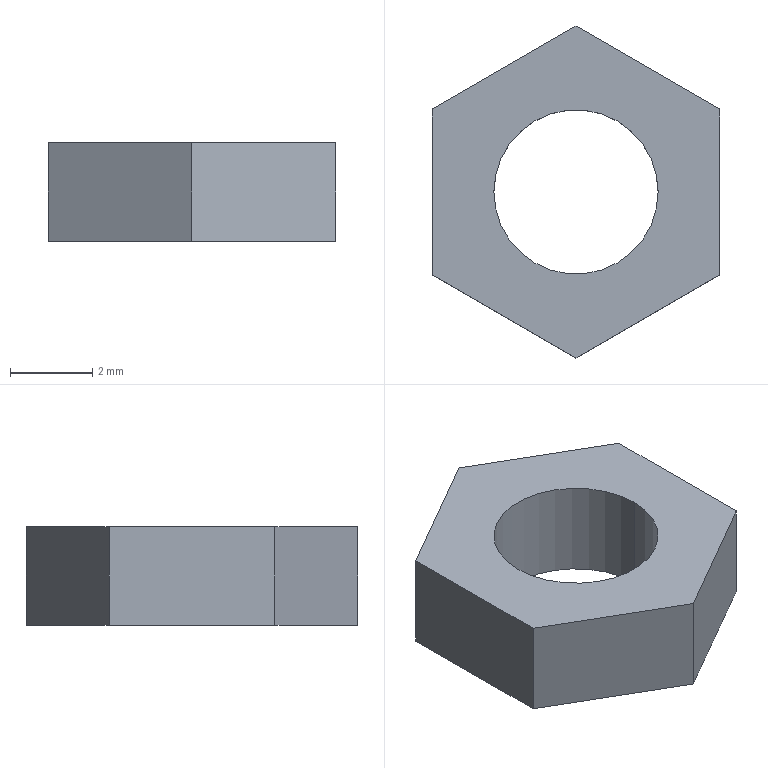Part | STEP file | M4 nut | 1 solid | 10 faces | box 7 x 8.083 x 2.4 mm | volume 71.685 mm3 | plane 8 | cylinder 2 | commonest cylinder face diameters 4 x2
STEP:
#1=CARTESIAN_POINT('',(0.,0.,0.));
#2=DIRECTION('',(0.,0.,1.));
#3=DIRECTION('',(1.,0.,0.));
#4=AXIS2_PLACEMENT_3D('',#1,#2,#3);
#5=CARTESIAN_POINT('',(2.,0.,0.));
#6=VERTEX_POINT('',#5);
#7=CARTESIAN_POINT('',(2.,0.,2.4));
#8=VERTEX_POINT('',#7);
#9=CARTESIAN_POINT('',(2.,0.,0.));
#10=DIRECTION('',(0.,0.,1.));
#11=VECTOR('',#10,1.);
#12=LINE('',#9,#11);
#13=CARTESIAN_POINT('',(0.,0.,0.));
#14=DIRECTION('',(0.,0.,1.));
#15=DIRECTION('',(1.,0.,0.));
#16=AXIS2_PLACEMENT_3D('',#13,#14,#15);
#17=CYLINDRICAL_SURFACE('',#16,2.);
#18=CARTESIAN_POINT('',(6.283,0.));
#19=DIRECTION('',(0.,1.));
#20=VECTOR('',#19,1.);
#21=LINE('',#18,#20);
#22=(GEOMETRIC_REPRESENTATION_CONTEXT(2)PARAMETRIC_REPRESENTATION_CONTEXT()REPRESENTATION_CONTEXT('',''));
#23=DEFINITIONAL_REPRESENTATION('',(#21),#22);
#24=PCURVE('',#17,#23);
#25=CARTESIAN_POINT('',(0.,0.,0.));
#26=DIRECTION('',(0.,0.,1.));
#27=DIRECTION('',(1.,0.,0.));
#28=AXIS2_PLACEMENT_3D('',#25,#26,#27);
#29=CYLINDRICAL_SURFACE('',#28,2.);
#30=CARTESIAN_POINT('',(0.,0.));
#31=DIRECTION('',(0.,1.));
#32=VECTOR('',#31,1.);
#33=LINE('',#30,#32);
#34=(GEOMETRIC_REPRESENTATION_CONTEXT(2)PARAMETRIC_REPRESENTATION_CONTEXT()REPRESENTATION_CONTEXT('',''));
#35=DEFINITIONAL_REPRESENTATION('',(#33),#34);
#36=PCURVE('',#29,#35);
#37=SURFACE_CURVE('',#12,(#24,#36),.PCURVE_S1.);
#38=EDGE_CURVE('',#6,#8,#37,.T.);
#39=ORIENTED_EDGE('',*,*,#38,.T.);
#40=CARTESIAN_POINT('',(-2.,0.,2.4));
#41=VERTEX_POINT('',#40);
#42=CARTESIAN_POINT('',(0.,0.,2.4));
#43=DIRECTION('',(0.,0.,1.));
#44=DIRECTION('',(1.,0.,0.));
#45=AXIS2_PLACEMENT_3D('',#42,#43,#44);
#46=CIRCLE('',#45,2.);
#47=CARTESIAN_POINT('',(0.,2.4));
#48=DIRECTION('',(1.,0.));
#49=VECTOR('',#48,1.);
#50=LINE('',#47,#49);
#51=(GEOMETRIC_REPRESENTATION_CONTEXT(2)PARAMETRIC_REPRESENTATION_CONTEXT()REPRESENTATION_CONTEXT('',''));
#52=DEFINITIONAL_REPRESENTATION('',(#50),#51);
#53=PCURVE('',#17,#52);
#54=CARTESIAN_POINT('',(0.,0.,2.4));
#55=DIRECTION('',(0.,0.,1.));
#56=DIRECTION('',(1.,0.,0.));
#57=AXIS2_PLACEMENT_3D('',#54,#55,#56);
#58=PLANE('',#57);
#59=CARTESIAN_POINT('',(0.,0.));
#60=DIRECTION('',(1.,0.));
#61=AXIS2_PLACEMENT_2D('',#59,#60);
#62=CIRCLE('',#61,2.);
#63=(GEOMETRIC_REPRESENTATION_CONTEXT(2)PARAMETRIC_REPRESENTATION_CONTEXT()REPRESENTATION_CONTEXT('',''));
#64=DEFINITIONAL_REPRESENTATION('',(#62),#63);
#65=PCURVE('',#58,#64);
#66=SURFACE_CURVE('',#46,(#53,#65),.PCURVE_S1.);
#67=EDGE_CURVE('',#41,#8,#66,.T.);
#68=ORIENTED_EDGE('',*,*,#67,.F.);
#69=CARTESIAN_POINT('',(-2.,0.,0.));
#70=VERTEX_POINT('',#69);
#71=CARTESIAN_POINT('',(-2.,0.,0.));
#72=DIRECTION('',(0.,0.,1.));
#73=VECTOR('',#72,1.);
#74=LINE('',#71,#73);
#75=CARTESIAN_POINT('',(3.142,0.));
#76=DIRECTION('',(0.,1.));
#77=VECTOR('',#76,1.);
#78=LINE('',#75,#77);
#79=(GEOMETRIC_REPRESENTATION_CONTEXT(2)PARAMETRIC_REPRESENTATION_CONTEXT()REPRESENTATION_CONTEXT('',''));
#80=DEFINITIONAL_REPRESENTATION('',(#78),#79);
#81=PCURVE('',#17,#80);
#82=CARTESIAN_POINT('',(3.142,0.));
#83=DIRECTION('',(0.,1.));
#84=VECTOR('',#83,1.);
#85=LINE('',#82,#84);
#86=(GEOMETRIC_REPRESENTATION_CONTEXT(2)PARAMETRIC_REPRESENTATION_CONTEXT()REPRESENTATION_CONTEXT('',''));
#87=DEFINITIONAL_REPRESENTATION('',(#85),#86);
#88=PCURVE('',#29,#87);
#89=SURFACE_CURVE('',#74,(#81,#88),.PCURVE_S1.);
#90=EDGE_CURVE('',#70,#41,#89,.T.);
#91=ORIENTED_EDGE('',*,*,#90,.F.);
#92=CARTESIAN_POINT('',(0.,0.,0.));
#93=DIRECTION('',(0.,0.,1.));
#94=DIRECTION('',(1.,0.,0.));
#95=AXIS2_PLACEMENT_3D('',#92,#93,#94);
#96=CIRCLE('',#95,2.);
#97=CARTESIAN_POINT('',(0.,0.));
#98=DIRECTION('',(1.,0.));
#99=VECTOR('',#98,1.);
#100=LINE('',#97,#99);
#101=(GEOMETRIC_REPRESENTATION_CONTEXT(2)PARAMETRIC_REPRESENTATION_CONTEXT()REPRESENTATION_CONTEXT('',''));
#102=DEFINITIONAL_REPRESENTATION('',(#100),#101);
#103=PCURVE('',#17,#102);
#104=CARTESIAN_POINT('',(0.,0.,0.));
#105=DIRECTION('',(0.,0.,1.));
#106=DIRECTION('',(1.,0.,0.));
#107=AXIS2_PLACEMENT_3D('',#104,#105,#106);
#108=PLANE('',#107);
#109=CARTESIAN_POINT('',(0.,0.));
#110=DIRECTION('',(1.,0.));
#111=AXIS2_PLACEMENT_2D('',#109,#110);
#112=CIRCLE('',#111,2.);
#113=(GEOMETRIC_REPRESENTATION_CONTEXT(2)PARAMETRIC_REPRESENTATION_CONTEXT()REPRESENTATION_CONTEXT('',''));
#114=DEFINITIONAL_REPRESENTATION('',(#112),#113);
#115=PCURVE('',#108,#114);
#116=SURFACE_CURVE('',#96,(#103,#115),.PCURVE_S1.);
#117=EDGE_CURVE('',#70,#6,#116,.T.);
#118=ORIENTED_EDGE('',*,*,#117,.T.);
#119=EDGE_LOOP('',(#39,#68,#91,#118));
#120=FACE_BOUND('',#119,.F.);
#121=ADVANCED_FACE('',(#120),#17,.F.);
#122=CARTESIAN_POINT('',(-3.5,2.021,0.));
#123=VERTEX_POINT('',#122);
#124=CARTESIAN_POINT('',(-3.5,-2.021,0.));
#125=VERTEX_POINT('',#124);
#126=CARTESIAN_POINT('',(-3.5,2.021,0.));
#127=DIRECTION('',(0.,-1.,0.));
#128=VECTOR('',#127,1.);
#129=LINE('',#126,#128);
#130=CARTESIAN_POINT('',(-3.5,2.021,2.4));
#131=DIRECTION('',(1.,0.,0.));
#132=DIRECTION('',(0.,1.,0.));
#133=AXIS2_PLACEMENT_3D('',#130,#131,#132);
#134=PLANE('',#133);
#135=CARTESIAN_POINT('',(0.,-2.4));
#136=DIRECTION('',(-1.,0.));
#137=VECTOR('',#136,1.);
#138=LINE('',#135,#137);
#139=(GEOMETRIC_REPRESENTATION_CONTEXT(2)PARAMETRIC_REPRESENTATION_CONTEXT()REPRESENTATION_CONTEXT('',''));
#140=DEFINITIONAL_REPRESENTATION('',(#138),#139);
#141=PCURVE('',#134,#140);
#142=CARTESIAN_POINT('',(-3.5,2.021));
#143=DIRECTION('',(0.,-1.));
#144=VECTOR('',#143,1.);
#145=LINE('',#142,#144);
#146=(GEOMETRIC_REPRESENTATION_CONTEXT(2)PARAMETRIC_REPRESENTATION_CONTEXT()REPRESENTATION_CONTEXT('',''));
#147=DEFINITIONAL_REPRESENTATION('',(#145),#146);
#148=PCURVE('',#108,#147);
#149=SURFACE_CURVE('',#129,(#141,#148),.PCURVE_S1.);
#150=EDGE_CURVE('',#123,#125,#149,.T.);
#151=ORIENTED_EDGE('',*,*,#150,.T.);
#152=CARTESIAN_POINT('',(-3.5,-2.021,2.4));
#153=VERTEX_POINT('',#152);
#154=CARTESIAN_POINT('',(-3.5,-2.021,2.4));
#155=DIRECTION('',(0.,0.,-1.));
#156=VECTOR('',#155,1.);
#157=LINE('',#154,#156);
#158=CARTESIAN_POINT('',(-4.041,0.));
#159=DIRECTION('',(0.,-1.));
#160=VECTOR('',#159,1.);
#161=LINE('',#158,#160);
#162=(GEOMETRIC_REPRESENTATION_CONTEXT(2)PARAMETRIC_REPRESENTATION_CONTEXT()REPRESENTATION_CONTEXT('',''));
#163=DEFINITIONAL_REPRESENTATION('',(#161),#162);
#164=PCURVE('',#134,#163);
#165=CARTESIAN_POINT('',(-3.5,-2.021,2.4));
#166=DIRECTION('',(0.5,0.866,0.));
#167=DIRECTION('',(-0.866,0.5,0.));
#168=AXIS2_PLACEMENT_3D('',#165,#166,#167);
#169=PLANE('',#168);
#170=CARTESIAN_POINT('',(0.,0.));
#171=DIRECTION('',(0.,-1.));
#172=VECTOR('',#171,1.);
#173=LINE('',#170,#172);
#174=(GEOMETRIC_REPRESENTATION_CONTEXT(2)PARAMETRIC_REPRESENTATION_CONTEXT()REPRESENTATION_CONTEXT('',''));
#175=DEFINITIONAL_REPRESENTATION('',(#173),#174);
#176=PCURVE('',#169,#175);
#177=SURFACE_CURVE('',#157,(#164,#176),.PCURVE_S1.);
#178=EDGE_CURVE('',#153,#125,#177,.T.);
#179=ORIENTED_EDGE('',*,*,#178,.F.);
#180=CARTESIAN_POINT('',(-3.5,2.021,2.4));
#181=VERTEX_POINT('',#180);
#182=CARTESIAN_POINT('',(-3.5,2.021,2.4));
#183=DIRECTION('',(0.,-1.,0.));
#184=VECTOR('',#183,1.);
#185=LINE('',#182,#184);
#186=CARTESIAN_POINT('',(0.,0.));
#187=DIRECTION('',(-1.,0.));
#188=VECTOR('',#187,1.);
#189=LINE('',#186,#188);
#190=(GEOMETRIC_REPRESENTATION_CONTEXT(2)PARAMETRIC_REPRESENTATION_CONTEXT()REPRESENTATION_CONTEXT('',''));
#191=DEFINITIONAL_REPRESENTATION('',(#189),#190);
#192=PCURVE('',#134,#191);
#193=CARTESIAN_POINT('',(-3.5,2.021));
#194=DIRECTION('',(0.,-1.));
#195=VECTOR('',#194,1.);
#196=LINE('',#193,#195);
#197=(GEOMETRIC_REPRESENTATION_CONTEXT(2)PARAMETRIC_REPRESENTATION_CONTEXT()REPRESENTATION_CONTEXT('',''));
#198=DEFINITIONAL_REPRESENTATION('',(#196),#197);
#199=PCURVE('',#58,#198);
#200=SURFACE_CURVE('',#185,(#192,#199),.PCURVE_S1.);
#201=EDGE_CURVE('',#181,#153,#200,.T.);
#202=ORIENTED_EDGE('',*,*,#201,.F.);
#203=CARTESIAN_POINT('',(-3.5,2.021,2.4));
#204=DIRECTION('',(0.,0.,-1.));
#205=VECTOR('',#204,1.);
#206=LINE('',#203,#205);
#207=CARTESIAN_POINT('',(0.,0.));
#208=DIRECTION('',(0.,-1.));
#209=VECTOR('',#208,1.);
#210=LINE('',#207,#209);
#211=(GEOMETRIC_REPRESENTATION_CONTEXT(2)PARAMETRIC_REPRESENTATION_CONTEXT()REPRESENTATION_CONTEXT('',''));
#212=DEFINITIONAL_REPRESENTATION('',(#210),#211);
#213=PCURVE('',#134,#212);
#214=CARTESIAN_POINT('',(0.,4.041,2.4));
#215=DIRECTION('',(0.5,-0.866,0.));
#216=DIRECTION('',(0.866,0.5,0.));
#217=AXIS2_PLACEMENT_3D('',#214,#215,#216);
#218=PLANE('',#217);
#219=CARTESIAN_POINT('',(-4.041,0.));
#220=DIRECTION('',(0.,-1.));
#221=VECTOR('',#220,1.);
#222=LINE('',#219,#221);
#223=(GEOMETRIC_REPRESENTATION_CONTEXT(2)PARAMETRIC_REPRESENTATION_CONTEXT()REPRESENTATION_CONTEXT('',''));
#224=DEFINITIONAL_REPRESENTATION('',(#222),#223);
#225=PCURVE('',#218,#224);
#226=SURFACE_CURVE('',#206,(#213,#225),.PCURVE_S1.);
#227=EDGE_CURVE('',#181,#123,#226,.T.);
#228=ORIENTED_EDGE('',*,*,#227,.T.);
#229=EDGE_LOOP('',(#151,#179,#202,#228));
#230=FACE_BOUND('',#229,.T.);
#231=ADVANCED_FACE('',(#230),#134,.F.);
#232=CARTESIAN_POINT('',(0.,-4.041,0.));
#233=VERTEX_POINT('',#232);
#234=CARTESIAN_POINT('',(-3.5,-2.021,0.));
#235=DIRECTION('',(0.866,-0.5,0.));
#236=VECTOR('',#235,1.);
#237=LINE('',#234,#236);
#238=CARTESIAN_POINT('',(0.,-2.4));
#239=DIRECTION('',(-1.,0.));
#240=VECTOR('',#239,1.);
#241=LINE('',#238,#240);
#242=(GEOMETRIC_REPRESENTATION_CONTEXT(2)PARAMETRIC_REPRESENTATION_CONTEXT()REPRESENTATION_CONTEXT('',''));
#243=DEFINITIONAL_REPRESENTATION('',(#241),#242);
#244=PCURVE('',#169,#243);
#245=CARTESIAN_POINT('',(-3.5,-2.021));
#246=DIRECTION('',(0.866,-0.5));
#247=VECTOR('',#246,1.);
#248=LINE('',#245,#247);
#249=(GEOMETRIC_REPRESENTATION_CONTEXT(2)PARAMETRIC_REPRESENTATION_CONTEXT()REPRESENTATION_CONTEXT('',''));
#250=DEFINITIONAL_REPRESENTATION('',(#248),#249);
#251=PCURVE('',#108,#250);
#252=SURFACE_CURVE('',#237,(#244,#251),.PCURVE_S1.);
#253=EDGE_CURVE('',#125,#233,#252,.T.);
#254=ORIENTED_EDGE('',*,*,#253,.T.);
#255=CARTESIAN_POINT('',(0.,-4.041,2.4));
#256=VERTEX_POINT('',#255);
#257=CARTESIAN_POINT('',(0.,-4.041,2.4));
#258=DIRECTION('',(0.,0.,-1.));
#259=VECTOR('',#258,1.);
#260=LINE('',#257,#259);
#261=CARTESIAN_POINT('',(-4.041,0.));
#262=DIRECTION('',(0.,-1.));
#263=VECTOR('',#262,1.);
#264=LINE('',#261,#263);
#265=(GEOMETRIC_REPRESENTATION_CONTEXT(2)PARAMETRIC_REPRESENTATION_CONTEXT()REPRESENTATION_CONTEXT('',''));
#266=DEFINITIONAL_REPRESENTATION('',(#264),#265);
#267=PCURVE('',#169,#266);
#268=CARTESIAN_POINT('',(0.,-4.041,2.4));
#269=DIRECTION('',(-0.5,0.866,0.));
#270=DIRECTION('',(-0.866,-0.5,0.));
#271=AXIS2_PLACEMENT_3D('',#268,#269,#270);
#272=PLANE('',#271);
#273=CARTESIAN_POINT('',(0.,0.));
#274=DIRECTION('',(0.,-1.));
#275=VECTOR('',#274,1.);
#276=LINE('',#273,#275);
#277=(GEOMETRIC_REPRESENTATION_CONTEXT(2)PARAMETRIC_REPRESENTATION_CONTEXT()REPRESENTATION_CONTEXT('',''));
#278=DEFINITIONAL_REPRESENTATION('',(#276),#277);
#279=PCURVE('',#272,#278);
#280=SURFACE_CURVE('',#260,(#267,#279),.PCURVE_S1.);
#281=EDGE_CURVE('',#256,#233,#280,.T.);
#282=ORIENTED_EDGE('',*,*,#281,.F.);
#283=CARTESIAN_POINT('',(-3.5,-2.021,2.4));
#284=DIRECTION('',(0.866,-0.5,0.));
#285=VECTOR('',#284,1.);
#286=LINE('',#283,#285);
#287=CARTESIAN_POINT('',(0.,0.));
#288=DIRECTION('',(-1.,0.));
#289=VECTOR('',#288,1.);
#290=LINE('',#287,#289);
#291=(GEOMETRIC_REPRESENTATION_CONTEXT(2)PARAMETRIC_REPRESENTATION_CONTEXT()REPRESENTATION_CONTEXT('',''));
#292=DEFINITIONAL_REPRESENTATION('',(#290),#291);
#293=PCURVE('',#169,#292);
#294=CARTESIAN_POINT('',(-3.5,-2.021));
#295=DIRECTION('',(0.866,-0.5));
#296=VECTOR('',#295,1.);
#297=LINE('',#294,#296);
#298=(GEOMETRIC_REPRESENTATION_CONTEXT(2)PARAMETRIC_REPRESENTATION_CONTEXT()REPRESENTATION_CONTEXT('',''));
#299=DEFINITIONAL_REPRESENTATION('',(#297),#298);
#300=PCURVE('',#58,#299);
#301=SURFACE_CURVE('',#286,(#293,#300),.PCURVE_S1.);
#302=EDGE_CURVE('',#153,#256,#301,.T.);
#303=ORIENTED_EDGE('',*,*,#302,.F.);
#304=ORIENTED_EDGE('',*,*,#178,.T.);
#305=EDGE_LOOP('',(#254,#282,#303,#304));
#306=FACE_BOUND('',#305,.T.);
#307=ADVANCED_FACE('',(#306),#169,.F.);
#308=CARTESIAN_POINT('',(3.5,-2.021,0.));
#309=VERTEX_POINT('',#308);
#310=CARTESIAN_POINT('',(0.,-4.041,0.));
#311=DIRECTION('',(0.866,0.5,0.));
#312=VECTOR('',#311,1.);
#313=LINE('',#310,#312);
#314=CARTESIAN_POINT('',(0.,-2.4));
#315=DIRECTION('',(-1.,0.));
#316=VECTOR('',#315,1.);
#317=LINE('',#314,#316);
#318=(GEOMETRIC_REPRESENTATION_CONTEXT(2)PARAMETRIC_REPRESENTATION_CONTEXT()REPRESENTATION_CONTEXT('',''));
#319=DEFINITIONAL_REPRESENTATION('',(#317),#318);
#320=PCURVE('',#272,#319);
#321=CARTESIAN_POINT('',(0.,-4.041));
#322=DIRECTION('',(0.866,0.5));
#323=VECTOR('',#322,1.);
#324=LINE('',#321,#323);
#325=(GEOMETRIC_REPRESENTATION_CONTEXT(2)PARAMETRIC_REPRESENTATION_CONTEXT()REPRESENTATION_CONTEXT('',''));
#326=DEFINITIONAL_REPRESENTATION('',(#324),#325);
#327=PCURVE('',#108,#326);
#328=SURFACE_CURVE('',#313,(#320,#327),.PCURVE_S1.);
#329=EDGE_CURVE('',#233,#309,#328,.T.);
#330=ORIENTED_EDGE('',*,*,#329,.T.);
#331=CARTESIAN_POINT('',(3.5,-2.021,2.4));
#332=VERTEX_POINT('',#331);
#333=CARTESIAN_POINT('',(3.5,-2.021,2.4));
#334=DIRECTION('',(0.,0.,-1.));
#335=VECTOR('',#334,1.);
#336=LINE('',#333,#335);
#337=CARTESIAN_POINT('',(-4.041,0.));
#338=DIRECTION('',(0.,-1.));
#339=VECTOR('',#338,1.);
#340=LINE('',#337,#339);
#341=(GEOMETRIC_REPRESENTATION_CONTEXT(2)PARAMETRIC_REPRESENTATION_CONTEXT()REPRESENTATION_CONTEXT('',''));
#342=DEFINITIONAL_REPRESENTATION('',(#340),#341);
#343=PCURVE('',#272,#342);
#344=CARTESIAN_POINT('',(3.5,-2.021,2.4));
#345=DIRECTION('',(-1.,0.,0.));
#346=DIRECTION('',(0.,0.,1.));
#347=AXIS2_PLACEMENT_3D('',#344,#345,#346);
#348=PLANE('',#347);
#349=CARTESIAN_POINT('',(0.,0.));
#350=DIRECTION('',(-1.,0.));
#351=VECTOR('',#350,1.);
#352=LINE('',#349,#351);
#353=(GEOMETRIC_REPRESENTATION_CONTEXT(2)PARAMETRIC_REPRESENTATION_CONTEXT()REPRESENTATION_CONTEXT('',''));
#354=DEFINITIONAL_REPRESENTATION('',(#352),#353);
#355=PCURVE('',#348,#354);
#356=SURFACE_CURVE('',#336,(#343,#355),.PCURVE_S1.);
#357=EDGE_CURVE('',#332,#309,#356,.T.);
#358=ORIENTED_EDGE('',*,*,#357,.F.);
#359=CARTESIAN_POINT('',(0.,-4.041,2.4));
#360=DIRECTION('',(0.866,0.5,0.));
#361=VECTOR('',#360,1.);
#362=LINE('',#359,#361);
#363=CARTESIAN_POINT('',(0.,0.));
#364=DIRECTION('',(-1.,0.));
#365=VECTOR('',#364,1.);
#366=LINE('',#363,#365);
#367=(GEOMETRIC_REPRESENTATION_CONTEXT(2)PARAMETRIC_REPRESENTATION_CONTEXT()REPRESENTATION_CONTEXT('',''));
#368=DEFINITIONAL_REPRESENTATION('',(#366),#367);
#369=PCURVE('',#272,#368);
#370=CARTESIAN_POINT('',(0.,-4.041));
#371=DIRECTION('',(0.866,0.5));
#372=VECTOR('',#371,1.);
#373=LINE('',#370,#372);
#374=(GEOMETRIC_REPRESENTATION_CONTEXT(2)PARAMETRIC_REPRESENTATION_CONTEXT()REPRESENTATION_CONTEXT('',''));
#375=DEFINITIONAL_REPRESENTATION('',(#373),#374);
#376=PCURVE('',#58,#375);
#377=SURFACE_CURVE('',#362,(#369,#376),.PCURVE_S1.);
#378=EDGE_CURVE('',#256,#332,#377,.T.);
#379=ORIENTED_EDGE('',*,*,#378,.F.);
#380=ORIENTED_EDGE('',*,*,#281,.T.);
#381=EDGE_LOOP('',(#330,#358,#379,#380));
#382=FACE_BOUND('',#381,.T.);
#383=ADVANCED_FACE('',(#382),#272,.F.);
#384=CARTESIAN_POINT('',(3.5,2.021,0.));
#385=VERTEX_POINT('',#384);
#386=CARTESIAN_POINT('',(3.5,-2.021,0.));
#387=DIRECTION('',(0.,1.,0.));
#388=VECTOR('',#387,1.);
#389=LINE('',#386,#388);
#390=CARTESIAN_POINT('',(-2.4,0.));
#391=DIRECTION('',(0.,1.));
#392=VECTOR('',#391,1.);
#393=LINE('',#390,#392);
#394=(GEOMETRIC_REPRESENTATION_CONTEXT(2)PARAMETRIC_REPRESENTATION_CONTEXT()REPRESENTATION_CONTEXT('',''));
#395=DEFINITIONAL_REPRESENTATION('',(#393),#394);
#396=PCURVE('',#348,#395);
#397=CARTESIAN_POINT('',(3.5,-2.021));
#398=DIRECTION('',(0.,1.));
#399=VECTOR('',#398,1.);
#400=LINE('',#397,#399);
#401=(GEOMETRIC_REPRESENTATION_CONTEXT(2)PARAMETRIC_REPRESENTATION_CONTEXT()REPRESENTATION_CONTEXT('',''));
#402=DEFINITIONAL_REPRESENTATION('',(#400),#401);
#403=PCURVE('',#108,#402);
#404=SURFACE_CURVE('',#389,(#396,#403),.PCURVE_S1.);
#405=EDGE_CURVE('',#309,#385,#404,.T.);
#406=ORIENTED_EDGE('',*,*,#405,.T.);
#407=CARTESIAN_POINT('',(3.5,2.021,2.4));
#408=VERTEX_POINT('',#407);
#409=CARTESIAN_POINT('',(3.5,2.021,2.4));
#410=DIRECTION('',(0.,0.,-1.));
#411=VECTOR('',#410,1.);
#412=LINE('',#409,#411);
#413=CARTESIAN_POINT('',(0.,4.041));
#414=DIRECTION('',(-1.,0.));
#415=VECTOR('',#414,1.);
#416=LINE('',#413,#415);
#417=(GEOMETRIC_REPRESENTATION_CONTEXT(2)PARAMETRIC_REPRESENTATION_CONTEXT()REPRESENTATION_CONTEXT('',''));
#418=DEFINITIONAL_REPRESENTATION('',(#416),#417);
#419=PCURVE('',#348,#418);
#420=CARTESIAN_POINT('',(3.5,2.021,2.4));
#421=DIRECTION('',(-0.5,-0.866,0.));
#422=DIRECTION('',(0.866,-0.5,0.));
#423=AXIS2_PLACEMENT_3D('',#420,#421,#422);
#424=PLANE('',#423);
#425=CARTESIAN_POINT('',(0.,0.));
#426=DIRECTION('',(0.,-1.));
#427=VECTOR('',#426,1.);
#428=LINE('',#425,#427);
#429=(GEOMETRIC_REPRESENTATION_CONTEXT(2)PARAMETRIC_REPRESENTATION_CONTEXT()REPRESENTATION_CONTEXT('',''));
#430=DEFINITIONAL_REPRESENTATION('',(#428),#429);
#431=PCURVE('',#424,#430);
#432=SURFACE_CURVE('',#412,(#419,#431),.PCURVE_S1.);
#433=EDGE_CURVE('',#408,#385,#432,.T.);
#434=ORIENTED_EDGE('',*,*,#433,.F.);
#435=CARTESIAN_POINT('',(3.5,-2.021,2.4));
#436=DIRECTION('',(0.,1.,0.));
#437=VECTOR('',#436,1.);
#438=LINE('',#435,#437);
#439=CARTESIAN_POINT('',(0.,0.));
#440=DIRECTION('',(0.,1.));
#441=VECTOR('',#440,1.);
#442=LINE('',#439,#441);
#443=(GEOMETRIC_REPRESENTATION_CONTEXT(2)PARAMETRIC_REPRESENTATION_CONTEXT()REPRESENTATION_CONTEXT('',''));
#444=DEFINITIONAL_REPRESENTATION('',(#442),#443);
#445=PCURVE('',#348,#444);
#446=CARTESIAN_POINT('',(3.5,-2.021));
#447=DIRECTION('',(0.,1.));
#448=VECTOR('',#447,1.);
#449=LINE('',#446,#448);
#450=(GEOMETRIC_REPRESENTATION_CONTEXT(2)PARAMETRIC_REPRESENTATION_CONTEXT()REPRESENTATION_CONTEXT('',''));
#451=DEFINITIONAL_REPRESENTATION('',(#449),#450);
#452=PCURVE('',#58,#451);
#453=SURFACE_CURVE('',#438,(#445,#452),.PCURVE_S1.);
#454=EDGE_CURVE('',#332,#408,#453,.T.);
#455=ORIENTED_EDGE('',*,*,#454,.F.);
#456=ORIENTED_EDGE('',*,*,#357,.T.);
#457=EDGE_LOOP('',(#406,#434,#455,#456));
#458=FACE_BOUND('',#457,.T.);
#459=ADVANCED_FACE('',(#458),#348,.F.);
#460=CARTESIAN_POINT('',(0.,4.041,0.));
#461=VERTEX_POINT('',#460);
#462=CARTESIAN_POINT('',(3.5,2.021,0.));
#463=DIRECTION('',(-0.866,0.5,0.));
#464=VECTOR('',#463,1.);
#465=LINE('',#462,#464);
#466=CARTESIAN_POINT('',(0.,-2.4));
#467=DIRECTION('',(-1.,0.));
#468=VECTOR('',#467,1.);
#469=LINE('',#466,#468);
#470=(GEOMETRIC_REPRESENTATION_CONTEXT(2)PARAMETRIC_REPRESENTATION_CONTEXT()REPRESENTATION_CONTEXT('',''));
#471=DEFINITIONAL_REPRESENTATION('',(#469),#470);
#472=PCURVE('',#424,#471);
#473=CARTESIAN_POINT('',(3.5,2.021));
#474=DIRECTION('',(-0.866,0.5));
#475=VECTOR('',#474,1.);
#476=LINE('',#473,#475);
#477=(GEOMETRIC_REPRESENTATION_CONTEXT(2)PARAMETRIC_REPRESENTATION_CONTEXT()REPRESENTATION_CONTEXT('',''));
#478=DEFINITIONAL_REPRESENTATION('',(#476),#477);
#479=PCURVE('',#108,#478);
#480=SURFACE_CURVE('',#465,(#472,#479),.PCURVE_S1.);
#481=EDGE_CURVE('',#385,#461,#480,.T.);
#482=ORIENTED_EDGE('',*,*,#481,.T.);
#483=CARTESIAN_POINT('',(0.,4.041,2.4));
#484=VERTEX_POINT('',#483);
#485=CARTESIAN_POINT('',(0.,4.041,2.4));
#486=DIRECTION('',(0.,0.,-1.));
#487=VECTOR('',#486,1.);
#488=LINE('',#485,#487);
#489=CARTESIAN_POINT('',(-4.041,0.));
#490=DIRECTION('',(0.,-1.));
#491=VECTOR('',#490,1.);
#492=LINE('',#489,#491);
#493=(GEOMETRIC_REPRESENTATION_CONTEXT(2)PARAMETRIC_REPRESENTATION_CONTEXT()REPRESENTATION_CONTEXT('',''));
#494=DEFINITIONAL_REPRESENTATION('',(#492),#493);
#495=PCURVE('',#424,#494);
#496=CARTESIAN_POINT('',(0.,0.));
#497=DIRECTION('',(0.,-1.));
#498=VECTOR('',#497,1.);
#499=LINE('',#496,#498);
#500=(GEOMETRIC_REPRESENTATION_CONTEXT(2)PARAMETRIC_REPRESENTATION_CONTEXT()REPRESENTATION_CONTEXT('',''));
#501=DEFINITIONAL_REPRESENTATION('',(#499),#500);
#502=PCURVE('',#218,#501);
#503=SURFACE_CURVE('',#488,(#495,#502),.PCURVE_S1.);
#504=EDGE_CURVE('',#484,#461,#503,.T.);
#505=ORIENTED_EDGE('',*,*,#504,.F.);
#506=CARTESIAN_POINT('',(3.5,2.021,2.4));
#507=DIRECTION('',(-0.866,0.5,0.));
#508=VECTOR('',#507,1.);
#509=LINE('',#506,#508);
#510=CARTESIAN_POINT('',(0.,0.));
#511=DIRECTION('',(-1.,0.));
#512=VECTOR('',#511,1.);
#513=LINE('',#510,#512);
#514=(GEOMETRIC_REPRESENTATION_CONTEXT(2)PARAMETRIC_REPRESENTATION_CONTEXT()REPRESENTATION_CONTEXT('',''));
#515=DEFINITIONAL_REPRESENTATION('',(#513),#514);
#516=PCURVE('',#424,#515);
#517=CARTESIAN_POINT('',(3.5,2.021));
#518=DIRECTION('',(-0.866,0.5));
#519=VECTOR('',#518,1.);
#520=LINE('',#517,#519);
#521=(GEOMETRIC_REPRESENTATION_CONTEXT(2)PARAMETRIC_REPRESENTATION_CONTEXT()REPRESENTATION_CONTEXT('',''));
#522=DEFINITIONAL_REPRESENTATION('',(#520),#521);
#523=PCURVE('',#58,#522);
#524=SURFACE_CURVE('',#509,(#516,#523),.PCURVE_S1.);
#525=EDGE_CURVE('',#408,#484,#524,.T.);
#526=ORIENTED_EDGE('',*,*,#525,.F.);
#527=ORIENTED_EDGE('',*,*,#433,.T.);
#528=EDGE_LOOP('',(#482,#505,#526,#527));
#529=FACE_BOUND('',#528,.T.);
#530=ADVANCED_FACE('',(#529),#424,.F.);
#531=CARTESIAN_POINT('',(0.,4.041,0.));
#532=DIRECTION('',(-0.866,-0.5,0.));
#533=VECTOR('',#532,1.);
#534=LINE('',#531,#533);
#535=CARTESIAN_POINT('',(0.,-2.4));
#536=DIRECTION('',(-1.,0.));
#537=VECTOR('',#536,1.);
#538=LINE('',#535,#537);
#539=(GEOMETRIC_REPRESENTATION_CONTEXT(2)PARAMETRIC_REPRESENTATION_CONTEXT()REPRESENTATION_CONTEXT('',''));
#540=DEFINITIONAL_REPRESENTATION('',(#538),#539);
#541=PCURVE('',#218,#540);
#542=CARTESIAN_POINT('',(0.,4.041));
#543=DIRECTION('',(-0.866,-0.5));
#544=VECTOR('',#543,1.);
#545=LINE('',#542,#544);
#546=(GEOMETRIC_REPRESENTATION_CONTEXT(2)PARAMETRIC_REPRESENTATION_CONTEXT()REPRESENTATION_CONTEXT('',''));
#547=DEFINITIONAL_REPRESENTATION('',(#545),#546);
#548=PCURVE('',#108,#547);
#549=SURFACE_CURVE('',#534,(#541,#548),.PCURVE_S1.);
#550=EDGE_CURVE('',#461,#123,#549,.T.);
#551=ORIENTED_EDGE('',*,*,#550,.T.);
#552=ORIENTED_EDGE('',*,*,#227,.F.);
#553=CARTESIAN_POINT('',(0.,4.041,2.4));
#554=DIRECTION('',(-0.866,-0.5,0.));
#555=VECTOR('',#554,1.);
#556=LINE('',#553,#555);
#557=CARTESIAN_POINT('',(0.,0.));
#558=DIRECTION('',(-1.,0.));
#559=VECTOR('',#558,1.);
#560=LINE('',#557,#559);
#561=(GEOMETRIC_REPRESENTATION_CONTEXT(2)PARAMETRIC_REPRESENTATION_CONTEXT()REPRESENTATION_CONTEXT('',''));
#562=DEFINITIONAL_REPRESENTATION('',(#560),#561);
#563=PCURVE('',#218,#562);
#564=CARTESIAN_POINT('',(0.,4.041));
#565=DIRECTION('',(-0.866,-0.5));
#566=VECTOR('',#565,1.);
#567=LINE('',#564,#566);
#568=(GEOMETRIC_REPRESENTATION_CONTEXT(2)PARAMETRIC_REPRESENTATION_CONTEXT()REPRESENTATION_CONTEXT('',''));
#569=DEFINITIONAL_REPRESENTATION('',(#567),#568);
#570=PCURVE('',#58,#569);
#571=SURFACE_CURVE('',#556,(#563,#570),.PCURVE_S1.);
#572=EDGE_CURVE('',#484,#181,#571,.T.);
#573=ORIENTED_EDGE('',*,*,#572,.F.);
#574=ORIENTED_EDGE('',*,*,#504,.T.);
#575=EDGE_LOOP('',(#551,#552,#573,#574));
#576=FACE_BOUND('',#575,.T.);
#577=ADVANCED_FACE('',(#576),#218,.F.);
#578=CARTESIAN_POINT('',(0.,0.,2.4));
#579=DIRECTION('',(0.,0.,1.));
#580=DIRECTION('',(1.,0.,0.));
#581=AXIS2_PLACEMENT_3D('',#578,#579,#580);
#582=CIRCLE('',#581,2.);
#583=CARTESIAN_POINT('',(0.,0.));
#584=DIRECTION('',(1.,0.));
#585=AXIS2_PLACEMENT_2D('',#583,#584);
#586=CIRCLE('',#585,2.);
#587=(GEOMETRIC_REPRESENTATION_CONTEXT(2)PARAMETRIC_REPRESENTATION_CONTEXT()REPRESENTATION_CONTEXT('',''));
#588=DEFINITIONAL_REPRESENTATION('',(#586),#587);
#589=PCURVE('',#58,#588);
#590=CARTESIAN_POINT('',(0.,2.4));
#591=DIRECTION('',(1.,0.));
#592=VECTOR('',#591,1.);
#593=LINE('',#590,#592);
#594=(GEOMETRIC_REPRESENTATION_CONTEXT(2)PARAMETRIC_REPRESENTATION_CONTEXT()REPRESENTATION_CONTEXT('',''));
#595=DEFINITIONAL_REPRESENTATION('',(#593),#594);
#596=PCURVE('',#29,#595);
#597=SURFACE_CURVE('',#582,(#589,#596),.PCURVE_S1.);
#598=EDGE_CURVE('',#8,#41,#597,.T.);
#599=ORIENTED_EDGE('',*,*,#598,.F.);
#600=ORIENTED_EDGE('',*,*,#67,.F.);
#601=EDGE_LOOP('',(#599,#600));
#602=FACE_BOUND('',#601,.T.);
#603=ORIENTED_EDGE('',*,*,#201,.T.);
#604=ORIENTED_EDGE('',*,*,#302,.T.);
#605=ORIENTED_EDGE('',*,*,#378,.T.);
#606=ORIENTED_EDGE('',*,*,#454,.T.);
#607=ORIENTED_EDGE('',*,*,#525,.T.);
#608=ORIENTED_EDGE('',*,*,#572,.T.);
#609=EDGE_LOOP('',(#603,#604,#605,#606,#607,#608));
#610=FACE_BOUND('',#609,.T.);
#611=ADVANCED_FACE('',(#602,#610),#58,.T.);
#612=CARTESIAN_POINT('',(0.,0.,0.));
#613=DIRECTION('',(0.,0.,1.));
#614=DIRECTION('',(1.,0.,0.));
#615=AXIS2_PLACEMENT_3D('',#612,#613,#614);
#616=CIRCLE('',#615,2.);
#617=CARTESIAN_POINT('',(0.,0.));
#618=DIRECTION('',(1.,0.));
#619=AXIS2_PLACEMENT_2D('',#617,#618);
#620=CIRCLE('',#619,2.);
#621=(GEOMETRIC_REPRESENTATION_CONTEXT(2)PARAMETRIC_REPRESENTATION_CONTEXT()REPRESENTATION_CONTEXT('',''));
#622=DEFINITIONAL_REPRESENTATION('',(#620),#621);
#623=PCURVE('',#108,#622);
#624=CARTESIAN_POINT('',(0.,0.));
#625=DIRECTION('',(1.,0.));
#626=VECTOR('',#625,1.);
#627=LINE('',#624,#626);
#628=(GEOMETRIC_REPRESENTATION_CONTEXT(2)PARAMETRIC_REPRESENTATION_CONTEXT()REPRESENTATION_CONTEXT('',''));
#629=DEFINITIONAL_REPRESENTATION('',(#627),#628);
#630=PCURVE('',#29,#629);
#631=SURFACE_CURVE('',#616,(#623,#630),.PCURVE_S1.);
#632=EDGE_CURVE('',#6,#70,#631,.T.);
#633=ORIENTED_EDGE('',*,*,#632,.T.);
#634=ORIENTED_EDGE('',*,*,#117,.T.);
#635=EDGE_LOOP('',(#633,#634));
#636=FACE_BOUND('',#635,.T.);
#637=ORIENTED_EDGE('',*,*,#150,.F.);
#638=ORIENTED_EDGE('',*,*,#550,.F.);
#639=ORIENTED_EDGE('',*,*,#481,.F.);
#640=ORIENTED_EDGE('',*,*,#405,.F.);
#641=ORIENTED_EDGE('',*,*,#329,.F.);
#642=ORIENTED_EDGE('',*,*,#253,.F.);
#643=EDGE_LOOP('',(#637,#638,#639,#640,#641,#642));
#644=FACE_BOUND('',#643,.T.);
#645=ADVANCED_FACE('',(#636,#644),#108,.F.);
#646=ORIENTED_EDGE('',*,*,#598,.F.);
#647=ORIENTED_EDGE('',*,*,#38,.F.);
#648=ORIENTED_EDGE('',*,*,#632,.T.);
#649=ORIENTED_EDGE('',*,*,#90,.T.);
#650=EDGE_LOOP('',(#646,#647,#648,#649));
#651=FACE_BOUND('',#650,.F.);
#652=ADVANCED_FACE('',(#651),#29,.F.);
#653=CLOSED_SHELL('',(#121,#231,#307,#383,#459,#530,#577,#611,#645,#652));
#654=MANIFOLD_SOLID_BREP('',#653);
#655=(LENGTH_UNIT()NAMED_UNIT(*)SI_UNIT(.MILLI.,.METRE.));
#656=UNCERTAINTY_MEASURE_WITH_UNIT(LENGTH_MEASURE(0.0000001),#655,'','');
#657=(NAMED_UNIT(*)PLANE_ANGLE_UNIT()SI_UNIT($,.RADIAN.));
#658=(NAMED_UNIT(*)SI_UNIT($,.STERADIAN.)SOLID_ANGLE_UNIT());
#659=(GEOMETRIC_REPRESENTATION_CONTEXT(3)GLOBAL_UNCERTAINTY_ASSIGNED_CONTEXT((#656))GLOBAL_UNIT_ASSIGNED_CONTEXT((#655,#657,#658))REPRESENTATION_CONTEXT('',''));
#660=ADVANCED_BREP_SHAPE_REPRESENTATION('',(#4,#654),#659);